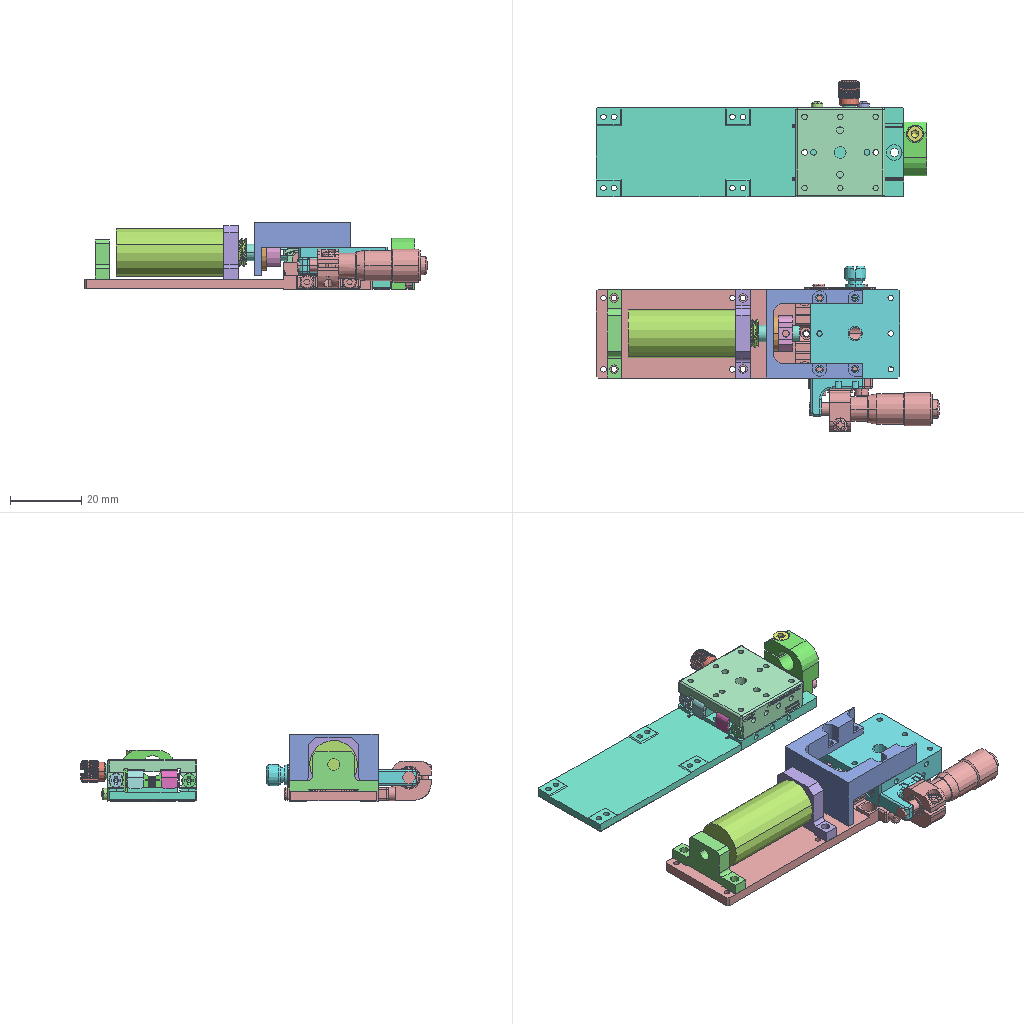Assembly | SolidWorks | 13 different items | 14 placed | box 96 x 99 x 19 mm
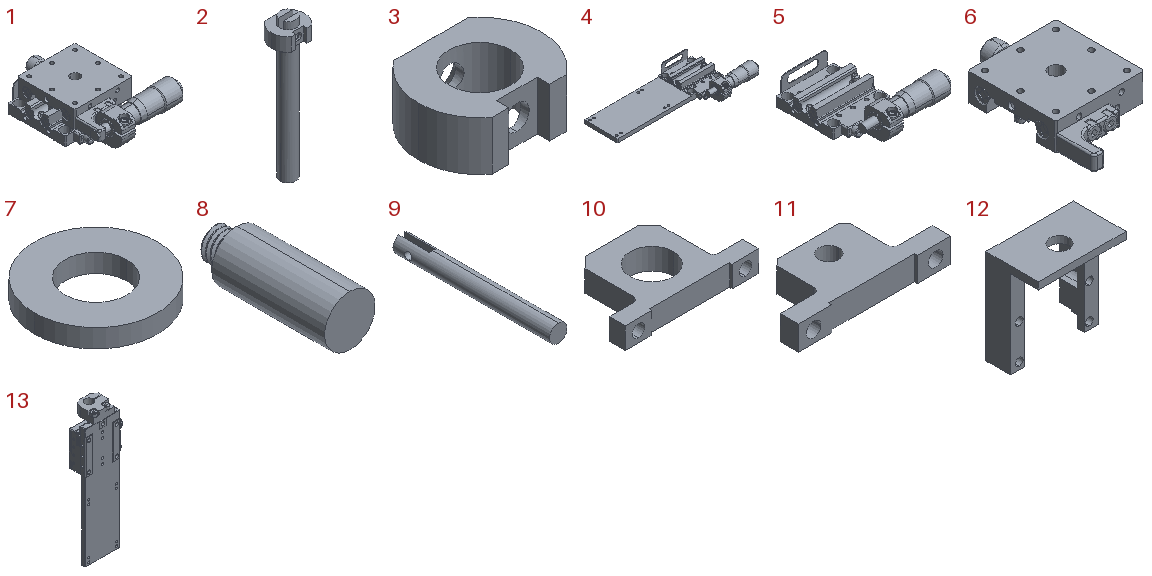Parts list (item | name | quantity | parent item | size | volume | features):
1 | (subassembly) | x1 | - | 40.495 x 46.4 x 12 mm | 8239 mm3 | -
2 | (subassembly) | x1 | - | 10 x 8 x 41.6 mm | 820.552 mm3 | -
3 | - | x1 | in 2 | 10 x 8 x 4 mm | 178.926 mm3 | features BaseBody 1
4 | - | x1 | - | 96.495 x 41.4 x 11.45 mm | 8301 mm3 | features ICE 5, HoleWzd 3, MoveFace 3, BaseBody 1, Chamfer 1, Cut 1, DelFace 1
5 | - | x1 | in 1 | 40.495 x 41.4 x 11.45 mm | 4555 mm3 | features BaseBody 1
6 | - | x1 | in 1 | - | - | features RefSurface 6, BaseBody 4
7 | - | x1 | - | 10 x 10 x 1.5 mm | 88.357 mm3 | features Extrusion 1
8 | - | x1 | - | 13.5 x 36.5 x 13.5 mm | 4034 mm3 | features BaseBody 1
9 | - | x1 | in 2 | 4.65 x 41.6 x 4.65 mm | 641.626 mm3 | features BaseBody 1
10 | - | x1 | - | 25 x 15 x 4 mm | 694.454 mm3 | features ICE 3, MoveFace 2, Chamfer 1, Cut 1, Extrusion 1, Fillet 1
11 | - | x2 | - | 25 x 11 x 4 mm | 592.362 mm3 | features ICE 2, MoveFace 2, Chamfer 1, Extrusion 1, Fillet 1, HoleWzd 1
12 | - | x1 | - | 25 x 15 x 27 mm | 1845 mm3 | features BaseBody 1
13 | - | x1 | - | - | - | features RefSurface 55
Mates (type | each side: item.copy, entity, surface, feature):
Coincident | 1.1 plane | assembly plane | 3 times
Coincident | 6.1 face plane Surface-Input 6 | 12.1 face plane Input 1
Concentric | 6.1 face cylinder Surface-Input 6 | 12.1 face cylinder Input 1 | 2 times
Concentric | 12.1 face cylinder Input 1 | 8.1 face cylinder Input 1
Concentric | 12.1 face cylinder Input 1 | 9.1 face cylinder Input 1
Concentric | 9.1 face cylinder Input 1 | 7.1 face cylinder Boss-Extrude1
Coincident | 12.1 face plane Input 1 | 7.1 face plane Boss-Extrude1
Coincident | 3.1 face plane Input 1 | 7.1 face plane Boss-Extrude1
Parallel | 12.1 face plane Input 1 | 3.1 face plane Input 1
Coincident | 4.1 face plane Input 1 | 5.1 face plane Input 1
Concentric | 4.1 face cylinder Input 1 | 5.1 face cylinder Input 1 | 2 times
Coincident | 4.1 face plane Cut-Extrude3 | 10.1 face plane Boss-Extrude1
DistanceDim | 10.1 face plane Boss-Extrude1 | 12.1 face plane Input 1
Coincident | 4.1 face plane Cut-Extrude3 | 11.1 face plane Boss-Extrude1
Coincident | 8.1 face plane Input 1 | 10.1 face plane Boss-Extrude1
Concentric | 8.1 face cylinder Input 1 | 11.1 edge
Concentric | 4.1 face cylinder M2 Tapped Hole2 | 11.1 face cylinder Cut-Extrude1 | 2 times
Concentric | 12.1 face cylinder Input 1 | 10.1 face cylinder Cut-Extrude1
Concentric | 8.1 face cylinder Input 1 | 11.1 face cylinder M4 Tapped Hole1
Coincident | 4.1 face plane Cut-Extrude3 | 11.2 face plane Boss-Extrude1
Concentric | 4.1 face cylinder M2 Tapped Hole3 | 11.2 face cylinder Cut-Extrude1